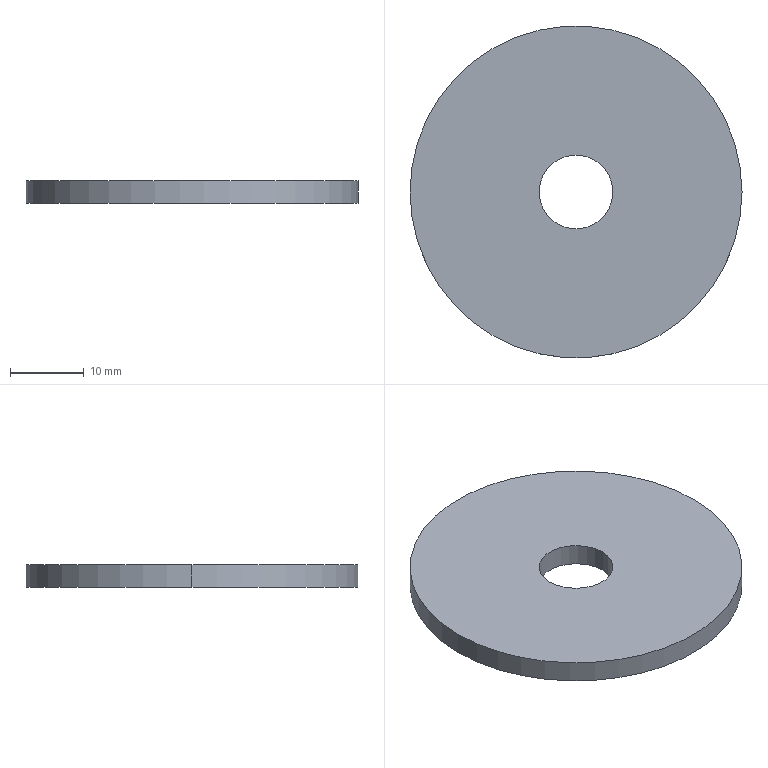Part | SolidWorks | features Extrusion 1 | 1 solid | 6 faces | box 45 x 45 x 3 mm | volume 4536 mm3 | cylinder 4 | plane 2 | commonest cylinder face diameters 10 x2 45 x2
STEP:
#1=CARTESIAN_POINT('',(-5.,0.,3.));
#2=VERTEX_POINT('',#1);
#3=CARTESIAN_POINT('',(5.,0.,3.));
#4=VERTEX_POINT('',#3);
#5=CARTESIAN_POINT('',(0.,0.,3.));
#6=DIRECTION('',(0.,0.,1.));
#7=DIRECTION('',(1.,0.,0.));
#8=AXIS2_PLACEMENT_3D('',#5,#6,#7);
#9=CIRCLE('',#8,5.);
#10=EDGE_CURVE('',#2,#4,#9,.T.);
#11=ORIENTED_EDGE('',*,*,#10,.T.);
#12=CARTESIAN_POINT('',(5.,0.,0.));
#13=VERTEX_POINT('',#12);
#14=CARTESIAN_POINT('',(5.,0.,3.));
#15=DIRECTION('',(0.,0.,-1.));
#16=VECTOR('',#15,1000.);
#17=LINE('',#14,#16);
#18=EDGE_CURVE('',#4,#13,#17,.T.);
#19=ORIENTED_EDGE('',*,*,#18,.T.);
#20=CARTESIAN_POINT('',(-5.,0.,0.));
#21=VERTEX_POINT('',#20);
#22=CARTESIAN_POINT('',(0.,0.,0.));
#23=DIRECTION('',(0.,0.,1.));
#24=DIRECTION('',(1.,0.,0.));
#25=AXIS2_PLACEMENT_3D('',#22,#23,#24);
#26=CIRCLE('',#25,5.);
#27=EDGE_CURVE('',#21,#13,#26,.T.);
#28=ORIENTED_EDGE('',*,*,#27,.F.);
#29=CARTESIAN_POINT('',(-5.,0.,3.));
#30=DIRECTION('',(0.,0.,-1.));
#31=VECTOR('',#30,1000.);
#32=LINE('',#29,#31);
#33=EDGE_CURVE('',#2,#21,#32,.T.);
#34=ORIENTED_EDGE('',*,*,#33,.F.);
#35=EDGE_LOOP('',(#11,#19,#28,#34));
#36=FACE_OUTER_BOUND('',#35,.T.);
#37=CARTESIAN_POINT('',(0.,0.,3.));
#38=DIRECTION('',(0.,0.,-1.));
#39=DIRECTION('',(-1.,0.,0.));
#40=AXIS2_PLACEMENT_3D('',#37,#38,#39);
#41=CYLINDRICAL_SURFACE('',#40,5.);
#42=ADVANCED_FACE('',(#36),#41,.F.);
#43=CARTESIAN_POINT('',(22.5,0.,3.));
#44=VERTEX_POINT('',#43);
#45=CARTESIAN_POINT('',(-22.5,0.,3.));
#46=VERTEX_POINT('',#45);
#47=CARTESIAN_POINT('',(0.,0.,3.));
#48=DIRECTION('',(0.,0.,1.));
#49=DIRECTION('',(1.,0.,0.));
#50=AXIS2_PLACEMENT_3D('',#47,#48,#49);
#51=CIRCLE('',#50,22.5);
#52=EDGE_CURVE('',#44,#46,#51,.T.);
#53=ORIENTED_EDGE('',*,*,#52,.F.);
#54=CARTESIAN_POINT('',(22.5,0.,0.));
#55=VERTEX_POINT('',#54);
#56=CARTESIAN_POINT('',(22.5,0.,3.));
#57=DIRECTION('',(0.,0.,-1.));
#58=VECTOR('',#57,1000.);
#59=LINE('',#56,#58);
#60=EDGE_CURVE('',#44,#55,#59,.T.);
#61=ORIENTED_EDGE('',*,*,#60,.T.);
#62=CARTESIAN_POINT('',(-22.5,0.,0.));
#63=VERTEX_POINT('',#62);
#64=CARTESIAN_POINT('',(0.,0.,0.));
#65=DIRECTION('',(0.,0.,1.));
#66=DIRECTION('',(1.,0.,0.));
#67=AXIS2_PLACEMENT_3D('',#64,#65,#66);
#68=CIRCLE('',#67,22.5);
#69=EDGE_CURVE('',#55,#63,#68,.T.);
#70=ORIENTED_EDGE('',*,*,#69,.T.);
#71=CARTESIAN_POINT('',(-22.5,0.,3.));
#72=DIRECTION('',(0.,0.,-1.));
#73=VECTOR('',#72,1000.);
#74=LINE('',#71,#73);
#75=EDGE_CURVE('',#46,#63,#74,.T.);
#76=ORIENTED_EDGE('',*,*,#75,.F.);
#77=EDGE_LOOP('',(#53,#61,#70,#76));
#78=FACE_OUTER_BOUND('',#77,.T.);
#79=CARTESIAN_POINT('',(0.,0.,3.));
#80=DIRECTION('',(0.,0.,-1.));
#81=DIRECTION('',(-1.,0.,0.));
#82=AXIS2_PLACEMENT_3D('',#79,#80,#81);
#83=CYLINDRICAL_SURFACE('',#82,22.5);
#84=ADVANCED_FACE('',(#78),#83,.T.);
#85=CARTESIAN_POINT('',(0.,0.,3.));
#86=DIRECTION('',(0.,0.,1.));
#87=DIRECTION('',(1.,0.,0.));
#88=AXIS2_PLACEMENT_3D('',#85,#86,#87);
#89=CIRCLE('',#88,22.5);
#90=EDGE_CURVE('',#46,#44,#89,.T.);
#91=ORIENTED_EDGE('',*,*,#90,.T.);
#92=ORIENTED_EDGE('',*,*,#52,.T.);
#93=EDGE_LOOP('',(#91,#92));
#94=FACE_OUTER_BOUND('',#93,.T.);
#95=ORIENTED_EDGE('',*,*,#10,.F.);
#96=CARTESIAN_POINT('',(0.,0.,3.));
#97=DIRECTION('',(0.,0.,1.));
#98=DIRECTION('',(1.,0.,0.));
#99=AXIS2_PLACEMENT_3D('',#96,#97,#98);
#100=CIRCLE('',#99,5.);
#101=EDGE_CURVE('',#4,#2,#100,.T.);
#102=ORIENTED_EDGE('',*,*,#101,.F.);
#103=EDGE_LOOP('',(#95,#102));
#104=FACE_BOUND('',#103,.T.);
#105=CARTESIAN_POINT('',(0.,0.,3.));
#106=DIRECTION('',(0.,0.,1.));
#107=DIRECTION('',(1.,0.,0.));
#108=AXIS2_PLACEMENT_3D('',#105,#106,#107);
#109=PLANE('',#108);
#110=ADVANCED_FACE('',(#94,#104),#109,.T.);
#111=CARTESIAN_POINT('',(0.,0.,0.));
#112=DIRECTION('',(0.,0.,1.));
#113=DIRECTION('',(1.,0.,0.));
#114=AXIS2_PLACEMENT_3D('',#111,#112,#113);
#115=CIRCLE('',#114,22.5);
#116=EDGE_CURVE('',#63,#55,#115,.T.);
#117=ORIENTED_EDGE('',*,*,#116,.F.);
#118=ORIENTED_EDGE('',*,*,#69,.F.);
#119=EDGE_LOOP('',(#117,#118));
#120=FACE_OUTER_BOUND('',#119,.T.);
#121=ORIENTED_EDGE('',*,*,#27,.T.);
#122=CARTESIAN_POINT('',(0.,0.,0.));
#123=DIRECTION('',(0.,0.,1.));
#124=DIRECTION('',(1.,0.,0.));
#125=AXIS2_PLACEMENT_3D('',#122,#123,#124);
#126=CIRCLE('',#125,5.);
#127=EDGE_CURVE('',#13,#21,#126,.T.);
#128=ORIENTED_EDGE('',*,*,#127,.T.);
#129=EDGE_LOOP('',(#121,#128));
#130=FACE_BOUND('',#129,.T.);
#131=CARTESIAN_POINT('',(0.,0.,0.));
#132=DIRECTION('',(0.,0.,1.));
#133=DIRECTION('',(1.,0.,0.));
#134=AXIS2_PLACEMENT_3D('',#131,#132,#133);
#135=PLANE('',#134);
#136=ADVANCED_FACE('',(#120,#130),#135,.F.);
#137=ORIENTED_EDGE('',*,*,#60,.F.);
#138=ORIENTED_EDGE('',*,*,#90,.F.);
#139=ORIENTED_EDGE('',*,*,#75,.T.);
#140=ORIENTED_EDGE('',*,*,#116,.T.);
#141=EDGE_LOOP('',(#137,#138,#139,#140));
#142=FACE_OUTER_BOUND('',#141,.T.);
#143=CARTESIAN_POINT('',(0.,0.,3.));
#144=DIRECTION('',(0.,0.,-1.));
#145=DIRECTION('',(-1.,0.,0.));
#146=AXIS2_PLACEMENT_3D('',#143,#144,#145);
#147=CYLINDRICAL_SURFACE('',#146,22.5);
#148=ADVANCED_FACE('',(#142),#147,.T.);
#149=ORIENTED_EDGE('',*,*,#18,.F.);
#150=ORIENTED_EDGE('',*,*,#101,.T.);
#151=ORIENTED_EDGE('',*,*,#33,.T.);
#152=ORIENTED_EDGE('',*,*,#127,.F.);
#153=EDGE_LOOP('',(#149,#150,#151,#152));
#154=FACE_OUTER_BOUND('',#153,.T.);
#155=CARTESIAN_POINT('',(0.,0.,3.));
#156=DIRECTION('',(0.,0.,-1.));
#157=DIRECTION('',(-1.,0.,0.));
#158=AXIS2_PLACEMENT_3D('',#155,#156,#157);
#159=CYLINDRICAL_SURFACE('',#158,5.);
#160=ADVANCED_FACE('',(#154),#159,.F.);
#161=CLOSED_SHELL('',(#42,#84,#110,#136,#148,#160));
#162=MANIFOLD_SOLID_BREP('',#161);
#163=CARTESIAN_POINT('',(0.,0.,0.));
#164=DIRECTION('',(0.,0.,1.));
#165=DIRECTION('',(1.,0.,0.));
#166=AXIS2_PLACEMENT_3D('',#163,#164,#165);
#167=(LENGTH_UNIT()NAMED_UNIT(*)SI_UNIT(.MILLI.,.METRE.));
#168=UNCERTAINTY_MEASURE_WITH_UNIT(LENGTH_MEASURE(0.00001),#167,'','');
#169=(NAMED_UNIT(*)PLANE_ANGLE_UNIT()SI_UNIT($,.RADIAN.));
#170=(NAMED_UNIT(*)SI_UNIT($,.STERADIAN.)SOLID_ANGLE_UNIT());
#171=(GEOMETRIC_REPRESENTATION_CONTEXT(3)GLOBAL_UNCERTAINTY_ASSIGNED_CONTEXT((#168))GLOBAL_UNIT_ASSIGNED_CONTEXT((#167,#169,#170))REPRESENTATION_CONTEXT('',''));
#172=ADVANCED_BREP_SHAPE_REPRESENTATION('',(#162,#166),#171);